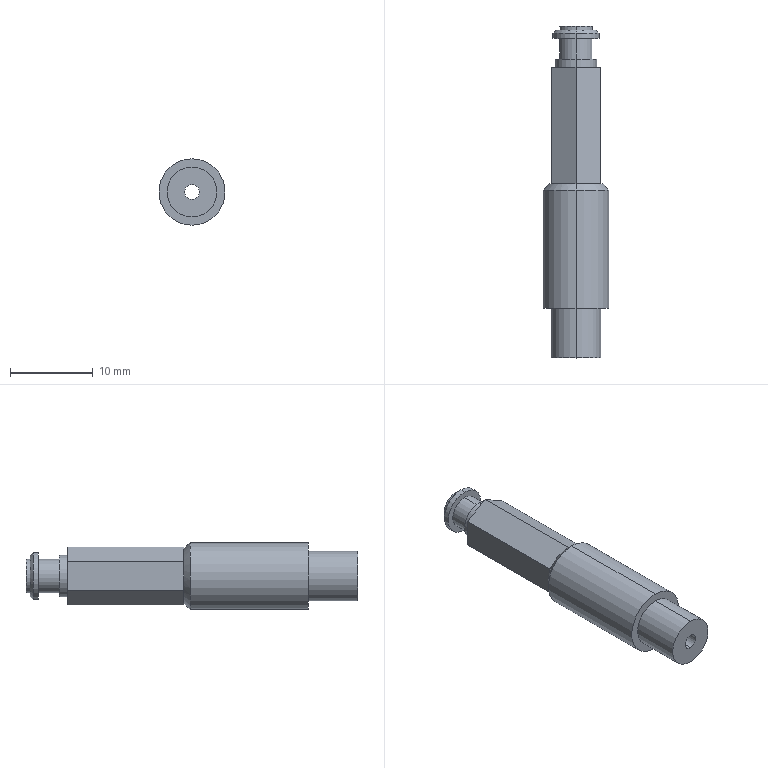Part | STEP file | PN_0031 | 1 solid | 43 faces | box 8 x 40 x 8 mm | volume 1332 mm3 | plane 25 | cylinder 14 | cone 4 | commonest cylinder face diameters 4 x4 1.8 x2 5 x2 5.6 x2 6 x2 8 x2